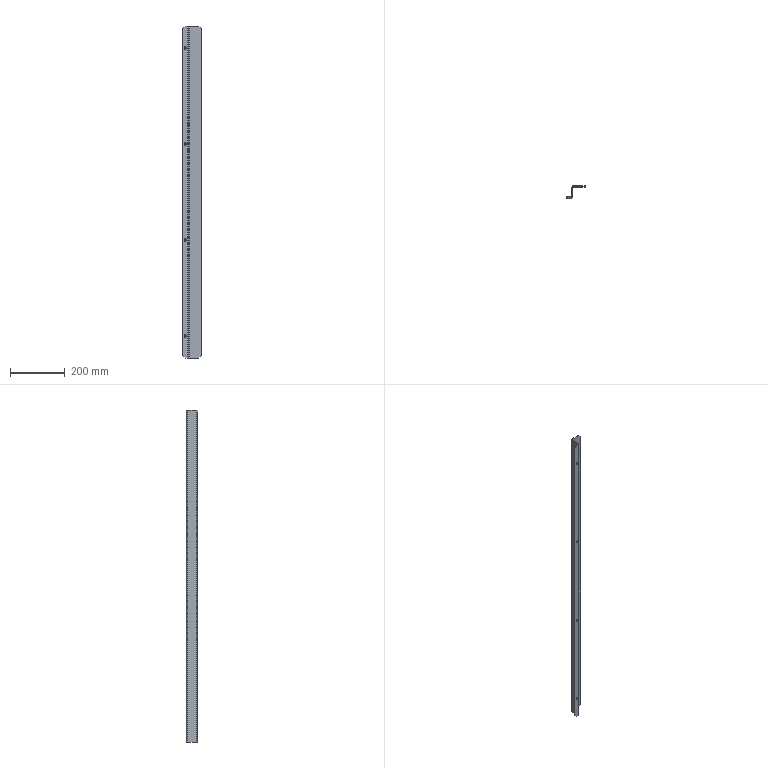Part | STEP file | HXGR200008-05-18 | 1 solid | 34 faces | box 70 x 42 x 1210 mm | volume 257088 mm3 | plane 22 | cylinder 12 | commonest cylinder face diameters 8 x8 6 x2 10 x2
STEP:
#1=CARTESIAN_POINT('',(10.,-2.,171.));
#2=VERTEX_POINT('',#1);
#3=CARTESIAN_POINT('',(10.,-2.,179.));
#4=VERTEX_POINT('',#3);
#5=CARTESIAN_POINT('',(10.,-2.,175.));
#6=DIRECTION('',(0.,1.,0.));
#7=DIRECTION('',(0.,0.,1.));
#8=AXIS2_PLACEMENT_3D('',#5,#6,#7);
#9=CIRCLE('',#8,4.);
#10=EDGE_CURVE('',#2,#4,#9,.T.);
#11=ORIENTED_EDGE('',*,*,#10,.F.);
#12=CARTESIAN_POINT('',(10.,0.,171.));
#13=VERTEX_POINT('',#12);
#14=CARTESIAN_POINT('',(10.,0.,171.));
#15=DIRECTION('',(0.,1.,0.));
#16=VECTOR('',#15,1000.);
#17=LINE('',#14,#16);
#18=EDGE_CURVE('',#2,#13,#17,.T.);
#19=ORIENTED_EDGE('',*,*,#18,.T.);
#20=CARTESIAN_POINT('',(10.,0.,179.));
#21=VERTEX_POINT('',#20);
#22=CARTESIAN_POINT('',(10.,0.,175.));
#23=DIRECTION('',(0.,1.,0.));
#24=DIRECTION('',(0.,0.,1.));
#25=AXIS2_PLACEMENT_3D('',#22,#23,#24);
#26=CIRCLE('',#25,4.);
#27=EDGE_CURVE('',#13,#21,#26,.T.);
#28=ORIENTED_EDGE('',*,*,#27,.T.);
#29=CARTESIAN_POINT('',(10.,0.,179.));
#30=DIRECTION('',(0.,1.,0.));
#31=VECTOR('',#30,1000.);
#32=LINE('',#29,#31);
#33=EDGE_CURVE('',#4,#21,#32,.T.);
#34=ORIENTED_EDGE('',*,*,#33,.F.);
#35=EDGE_LOOP('',(#11,#19,#28,#34));
#36=FACE_OUTER_BOUND('',#35,.T.);
#37=CARTESIAN_POINT('',(10.,0.,175.));
#38=DIRECTION('',(0.,1.,0.));
#39=DIRECTION('',(0.,0.,1.));
#40=AXIS2_PLACEMENT_3D('',#37,#38,#39);
#41=CYLINDRICAL_SURFACE('',#40,4.);
#42=ADVANCED_FACE('',(#36),#41,.F.);
#43=CARTESIAN_POINT('',(10.,-2.,-179.));
#44=VERTEX_POINT('',#43);
#45=CARTESIAN_POINT('',(10.,-2.,-171.));
#46=VERTEX_POINT('',#45);
#47=CARTESIAN_POINT('',(10.,-2.,-175.));
#48=DIRECTION('',(0.,1.,0.));
#49=DIRECTION('',(0.,0.,1.));
#50=AXIS2_PLACEMENT_3D('',#47,#48,#49);
#51=CIRCLE('',#50,4.);
#52=EDGE_CURVE('',#44,#46,#51,.T.);
#53=ORIENTED_EDGE('',*,*,#52,.F.);
#54=CARTESIAN_POINT('',(10.,0.,-179.));
#55=VERTEX_POINT('',#54);
#56=CARTESIAN_POINT('',(10.,0.,-179.));
#57=DIRECTION('',(0.,1.,0.));
#58=VECTOR('',#57,1000.);
#59=LINE('',#56,#58);
#60=EDGE_CURVE('',#44,#55,#59,.T.);
#61=ORIENTED_EDGE('',*,*,#60,.T.);
#62=CARTESIAN_POINT('',(10.,0.,-171.));
#63=VERTEX_POINT('',#62);
#64=CARTESIAN_POINT('',(10.,0.,-175.));
#65=DIRECTION('',(0.,1.,0.));
#66=DIRECTION('',(0.,0.,1.));
#67=AXIS2_PLACEMENT_3D('',#64,#65,#66);
#68=CIRCLE('',#67,4.);
#69=EDGE_CURVE('',#55,#63,#68,.T.);
#70=ORIENTED_EDGE('',*,*,#69,.T.);
#71=CARTESIAN_POINT('',(10.,0.,-171.));
#72=DIRECTION('',(0.,1.,0.));
#73=VECTOR('',#72,1000.);
#74=LINE('',#71,#73);
#75=EDGE_CURVE('',#46,#63,#74,.T.);
#76=ORIENTED_EDGE('',*,*,#75,.F.);
#77=EDGE_LOOP('',(#53,#61,#70,#76));
#78=FACE_OUTER_BOUND('',#77,.T.);
#79=CARTESIAN_POINT('',(10.,0.,-175.));
#80=DIRECTION('',(0.,1.,0.));
#81=DIRECTION('',(0.,0.,1.));
#82=AXIS2_PLACEMENT_3D('',#79,#80,#81);
#83=CYLINDRICAL_SURFACE('',#82,4.);
#84=ADVANCED_FACE('',(#78),#83,.F.);
#85=CARTESIAN_POINT('',(10.,-2.,521.));
#86=VERTEX_POINT('',#85);
#87=CARTESIAN_POINT('',(10.,-2.,529.));
#88=VERTEX_POINT('',#87);
#89=CARTESIAN_POINT('',(10.,-2.,525.));
#90=DIRECTION('',(0.,1.,0.));
#91=DIRECTION('',(0.,0.,1.));
#92=AXIS2_PLACEMENT_3D('',#89,#90,#91);
#93=CIRCLE('',#92,4.);
#94=EDGE_CURVE('',#86,#88,#93,.T.);
#95=ORIENTED_EDGE('',*,*,#94,.F.);
#96=CARTESIAN_POINT('',(10.,0.,521.));
#97=VERTEX_POINT('',#96);
#98=CARTESIAN_POINT('',(10.,0.,521.));
#99=DIRECTION('',(0.,1.,0.));
#100=VECTOR('',#99,1000.);
#101=LINE('',#98,#100);
#102=EDGE_CURVE('',#86,#97,#101,.T.);
#103=ORIENTED_EDGE('',*,*,#102,.T.);
#104=CARTESIAN_POINT('',(10.,0.,529.));
#105=VERTEX_POINT('',#104);
#106=CARTESIAN_POINT('',(10.,0.,525.));
#107=DIRECTION('',(0.,1.,0.));
#108=DIRECTION('',(0.,0.,1.));
#109=AXIS2_PLACEMENT_3D('',#106,#107,#108);
#110=CIRCLE('',#109,4.);
#111=EDGE_CURVE('',#97,#105,#110,.T.);
#112=ORIENTED_EDGE('',*,*,#111,.T.);
#113=CARTESIAN_POINT('',(10.,0.,529.));
#114=DIRECTION('',(0.,1.,0.));
#115=VECTOR('',#114,1000.);
#116=LINE('',#113,#115);
#117=EDGE_CURVE('',#88,#105,#116,.T.);
#118=ORIENTED_EDGE('',*,*,#117,.F.);
#119=EDGE_LOOP('',(#95,#103,#112,#118));
#120=FACE_OUTER_BOUND('',#119,.T.);
#121=CARTESIAN_POINT('',(10.,0.,525.));
#122=DIRECTION('',(0.,1.,0.));
#123=DIRECTION('',(0.,0.,1.));
#124=AXIS2_PLACEMENT_3D('',#121,#122,#123);
#125=CYLINDRICAL_SURFACE('',#124,4.);
#126=ADVANCED_FACE('',(#120),#125,.F.);
#127=CARTESIAN_POINT('',(10.,-2.,-529.));
#128=VERTEX_POINT('',#127);
#129=CARTESIAN_POINT('',(10.,-2.,-521.));
#130=VERTEX_POINT('',#129);
#131=CARTESIAN_POINT('',(10.,-2.,-525.));
#132=DIRECTION('',(0.,1.,0.));
#133=DIRECTION('',(0.,0.,1.));
#134=AXIS2_PLACEMENT_3D('',#131,#132,#133);
#135=CIRCLE('',#134,4.);
#136=EDGE_CURVE('',#128,#130,#135,.T.);
#137=ORIENTED_EDGE('',*,*,#136,.F.);
#138=CARTESIAN_POINT('',(10.,0.,-529.));
#139=VERTEX_POINT('',#138);
#140=CARTESIAN_POINT('',(10.,0.,-529.));
#141=DIRECTION('',(0.,1.,0.));
#142=VECTOR('',#141,1000.);
#143=LINE('',#140,#142);
#144=EDGE_CURVE('',#128,#139,#143,.T.);
#145=ORIENTED_EDGE('',*,*,#144,.T.);
#146=CARTESIAN_POINT('',(10.,0.,-521.));
#147=VERTEX_POINT('',#146);
#148=CARTESIAN_POINT('',(10.,0.,-525.));
#149=DIRECTION('',(0.,1.,0.));
#150=DIRECTION('',(0.,0.,1.));
#151=AXIS2_PLACEMENT_3D('',#148,#149,#150);
#152=CIRCLE('',#151,4.);
#153=EDGE_CURVE('',#139,#147,#152,.T.);
#154=ORIENTED_EDGE('',*,*,#153,.T.);
#155=CARTESIAN_POINT('',(10.,0.,-521.));
#156=DIRECTION('',(0.,1.,0.));
#157=VECTOR('',#156,1000.);
#158=LINE('',#155,#157);
#159=EDGE_CURVE('',#130,#147,#158,.T.);
#160=ORIENTED_EDGE('',*,*,#159,.F.);
#161=EDGE_LOOP('',(#137,#145,#154,#160));
#162=FACE_OUTER_BOUND('',#161,.T.);
#163=CARTESIAN_POINT('',(10.,0.,-525.));
#164=DIRECTION('',(0.,1.,0.));
#165=DIRECTION('',(0.,0.,1.));
#166=AXIS2_PLACEMENT_3D('',#163,#164,#165);
#167=CYLINDRICAL_SURFACE('',#166,4.);
#168=ADVANCED_FACE('',(#162),#167,.F.);
#169=CARTESIAN_POINT('',(20.,3.,605.));
#170=VERTEX_POINT('',#169);
#171=CARTESIAN_POINT('',(22.,3.,605.));
#172=VERTEX_POINT('',#171);
#173=CARTESIAN_POINT('',(20.,3.,605.));
#174=DIRECTION('',(1.,0.,0.));
#175=VECTOR('',#174,1000.);
#176=LINE('',#173,#175);
#177=EDGE_CURVE('',#170,#172,#176,.T.);
#178=ORIENTED_EDGE('',*,*,#177,.F.);
#179=CARTESIAN_POINT('',(17.,0.,605.));
#180=VERTEX_POINT('',#179);
#181=CARTESIAN_POINT('',(17.,3.,605.));
#182=DIRECTION('',(0.,0.,1.));
#183=DIRECTION('',(-1.,0.,0.));
#184=AXIS2_PLACEMENT_3D('',#181,#182,#183);
#185=CIRCLE('',#184,3.);
#186=EDGE_CURVE('',#180,#170,#185,.T.);
#187=ORIENTED_EDGE('',*,*,#186,.F.);
#188=CARTESIAN_POINT('',(17.,-2.,605.));
#189=VERTEX_POINT('',#188);
#190=CARTESIAN_POINT('',(17.,-2.,605.));
#191=DIRECTION('',(0.,1.,0.));
#192=VECTOR('',#191,1000.);
#193=LINE('',#190,#192);
#194=EDGE_CURVE('',#189,#180,#193,.T.);
#195=ORIENTED_EDGE('',*,*,#194,.F.);
#196=CARTESIAN_POINT('',(17.,3.,605.));
#197=DIRECTION('',(0.,0.,1.));
#198=DIRECTION('',(1.,0.,0.));
#199=AXIS2_PLACEMENT_3D('',#196,#197,#198);
#200=CIRCLE('',#199,5.);
#201=EDGE_CURVE('',#189,#172,#200,.T.);
#202=ORIENTED_EDGE('',*,*,#201,.T.);
#203=EDGE_LOOP('',(#178,#187,#195,#202));
#204=FACE_OUTER_BOUND('',#203,.T.);
#205=CARTESIAN_POINT('',(20.,3.,605.));
#206=DIRECTION('',(0.,0.,1.));
#207=DIRECTION('',(1.,0.,0.));
#208=AXIS2_PLACEMENT_3D('',#205,#206,#207);
#209=PLANE('',#208);
#210=ADVANCED_FACE('',(#204),#209,.T.);
#211=CARTESIAN_POINT('',(20.,35.,605.));
#212=VERTEX_POINT('',#211);
#213=CARTESIAN_POINT('',(20.,0.,605.));
#214=DIRECTION('',(0.,1.,0.));
#215=VECTOR('',#214,1000.);
#216=LINE('',#213,#215);
#217=EDGE_CURVE('',#170,#212,#216,.T.);
#218=ORIENTED_EDGE('',*,*,#217,.F.);
#219=ORIENTED_EDGE('',*,*,#177,.T.);
#220=CARTESIAN_POINT('',(22.,35.,605.));
#221=VERTEX_POINT('',#220);
#222=CARTESIAN_POINT('',(22.,0.,605.));
#223=DIRECTION('',(0.,1.,0.));
#224=VECTOR('',#223,1000.);
#225=LINE('',#222,#224);
#226=EDGE_CURVE('',#172,#221,#225,.T.);
#227=ORIENTED_EDGE('',*,*,#226,.T.);
#228=CARTESIAN_POINT('',(22.,35.,605.));
#229=DIRECTION('',(-1.,0.,0.));
#230=VECTOR('',#229,1000.);
#231=LINE('',#228,#230);
#232=EDGE_CURVE('',#221,#212,#231,.T.);
#233=ORIENTED_EDGE('',*,*,#232,.T.);
#234=EDGE_LOOP('',(#218,#219,#227,#233));
#235=FACE_OUTER_BOUND('',#234,.T.);
#236=CARTESIAN_POINT('',(17.,-2.,605.));
#237=DIRECTION('',(0.,0.,1.));
#238=DIRECTION('',(1.,0.,0.));
#239=AXIS2_PLACEMENT_3D('',#236,#237,#238);
#240=PLANE('',#239);
#241=ADVANCED_FACE('',(#235),#240,.T.);
#242=CARTESIAN_POINT('',(17.,0.,-605.));
#243=VERTEX_POINT('',#242);
#244=CARTESIAN_POINT('',(17.,-2.,-605.));
#245=VERTEX_POINT('',#244);
#246=CARTESIAN_POINT('',(17.,0.,-605.));
#247=DIRECTION('',(0.,-1.,0.));
#248=VECTOR('',#247,1000.);
#249=LINE('',#246,#248);
#250=EDGE_CURVE('',#243,#245,#249,.T.);
#251=ORIENTED_EDGE('',*,*,#250,.F.);
#252=CARTESIAN_POINT('',(20.,3.,-605.));
#253=VERTEX_POINT('',#252);
#254=CARTESIAN_POINT('',(17.,3.,-605.));
#255=DIRECTION('',(0.,0.,1.));
#256=DIRECTION('',(-1.,0.,0.));
#257=AXIS2_PLACEMENT_3D('',#254,#255,#256);
#258=CIRCLE('',#257,3.);
#259=EDGE_CURVE('',#243,#253,#258,.T.);
#260=ORIENTED_EDGE('',*,*,#259,.T.);
#261=CARTESIAN_POINT('',(22.,3.,-605.));
#262=VERTEX_POINT('',#261);
#263=CARTESIAN_POINT('',(22.,3.,-605.));
#264=DIRECTION('',(-1.,0.,0.));
#265=VECTOR('',#264,1000.);
#266=LINE('',#263,#265);
#267=EDGE_CURVE('',#262,#253,#266,.T.);
#268=ORIENTED_EDGE('',*,*,#267,.F.);
#269=CARTESIAN_POINT('',(17.,3.,-605.));
#270=DIRECTION('',(0.,0.,1.));
#271=DIRECTION('',(1.,0.,0.));
#272=AXIS2_PLACEMENT_3D('',#269,#270,#271);
#273=CIRCLE('',#272,5.);
#274=EDGE_CURVE('',#245,#262,#273,.T.);
#275=ORIENTED_EDGE('',*,*,#274,.F.);
#276=EDGE_LOOP('',(#251,#260,#268,#275));
#277=FACE_OUTER_BOUND('',#276,.T.);
#278=CARTESIAN_POINT('',(17.,0.,-605.));
#279=DIRECTION('',(0.,0.,-1.));
#280=DIRECTION('',(-1.,0.,0.));
#281=AXIS2_PLACEMENT_3D('',#278,#279,#280);
#282=PLANE('',#281);
#283=ADVANCED_FACE('',(#277),#282,.T.);
#284=CARTESIAN_POINT('',(10.,-2.,-605.));
#285=VERTEX_POINT('',#284);
#286=CARTESIAN_POINT('',(0.,-2.,-605.));
#287=DIRECTION('',(1.,0.,0.));
#288=VECTOR('',#287,1000.);
#289=LINE('',#286,#288);
#290=EDGE_CURVE('',#285,#245,#289,.T.);
#291=ORIENTED_EDGE('',*,*,#290,.F.);
#292=CARTESIAN_POINT('',(10.,0.,-605.));
#293=VERTEX_POINT('',#292);
#294=CARTESIAN_POINT('',(10.,3.,-605.));
#295=DIRECTION('',(0.,1.,0.));
#296=VECTOR('',#295,1000.);
#297=LINE('',#294,#296);
#298=EDGE_CURVE('',#285,#293,#297,.T.);
#299=ORIENTED_EDGE('',*,*,#298,.T.);
#300=CARTESIAN_POINT('',(0.,0.,-605.));
#301=DIRECTION('',(1.,0.,0.));
#302=VECTOR('',#301,1000.);
#303=LINE('',#300,#302);
#304=EDGE_CURVE('',#293,#243,#303,.T.);
#305=ORIENTED_EDGE('',*,*,#304,.T.);
#306=ORIENTED_EDGE('',*,*,#250,.T.);
#307=EDGE_LOOP('',(#291,#299,#305,#306));
#308=FACE_OUTER_BOUND('',#307,.T.);
#309=CARTESIAN_POINT('',(22.,3.,-605.));
#310=DIRECTION('',(0.,0.,-1.));
#311=DIRECTION('',(-1.,0.,0.));
#312=AXIS2_PLACEMENT_3D('',#309,#310,#311);
#313=PLANE('',#312);
#314=ADVANCED_FACE('',(#308),#313,.T.);
#315=CARTESIAN_POINT('',(25.,40.,605.));
#316=VERTEX_POINT('',#315);
#317=CARTESIAN_POINT('',(25.,38.,605.));
#318=VERTEX_POINT('',#317);
#319=CARTESIAN_POINT('',(25.,40.,605.));
#320=DIRECTION('',(0.,-1.,0.));
#321=VECTOR('',#320,1000.);
#322=LINE('',#319,#321);
#323=EDGE_CURVE('',#316,#318,#322,.T.);
#324=ORIENTED_EDGE('',*,*,#323,.F.);
#325=CARTESIAN_POINT('',(25.,35.,605.));
#326=DIRECTION('',(0.,0.,-1.));
#327=DIRECTION('',(1.,0.,0.));
#328=AXIS2_PLACEMENT_3D('',#325,#326,#327);
#329=CIRCLE('',#328,5.);
#330=EDGE_CURVE('',#212,#316,#329,.T.);
#331=ORIENTED_EDGE('',*,*,#330,.F.);
#332=ORIENTED_EDGE('',*,*,#232,.F.);
#333=CARTESIAN_POINT('',(25.,35.,605.));
#334=DIRECTION('',(0.,0.,-1.));
#335=DIRECTION('',(1.,0.,0.));
#336=AXIS2_PLACEMENT_3D('',#333,#334,#335);
#337=CIRCLE('',#336,3.);
#338=EDGE_CURVE('',#221,#318,#337,.T.);
#339=ORIENTED_EDGE('',*,*,#338,.T.);
#340=EDGE_LOOP('',(#324,#331,#332,#339));
#341=FACE_OUTER_BOUND('',#340,.T.);
#342=CARTESIAN_POINT('',(25.,40.,605.));
#343=DIRECTION('',(0.,0.,1.));
#344=DIRECTION('',(1.,0.,0.));
#345=AXIS2_PLACEMENT_3D('',#342,#343,#344);
#346=PLANE('',#345);
#347=ADVANCED_FACE('',(#341),#346,.T.);
#348=CARTESIAN_POINT('',(60.,38.,605.));
#349=VERTEX_POINT('',#348);
#350=CARTESIAN_POINT('',(20.,38.,605.));
#351=DIRECTION('',(1.,0.,0.));
#352=VECTOR('',#351,1000.);
#353=LINE('',#350,#352);
#354=EDGE_CURVE('',#318,#349,#353,.T.);
#355=ORIENTED_EDGE('',*,*,#354,.T.);
#356=CARTESIAN_POINT('',(60.,40.,605.));
#357=VERTEX_POINT('',#356);
#358=CARTESIAN_POINT('',(60.,35.,605.));
#359=DIRECTION('',(0.,1.,0.));
#360=VECTOR('',#359,1000.);
#361=LINE('',#358,#360);
#362=EDGE_CURVE('',#349,#357,#361,.T.);
#363=ORIENTED_EDGE('',*,*,#362,.T.);
#364=CARTESIAN_POINT('',(20.,40.,605.));
#365=DIRECTION('',(1.,0.,0.));
#366=VECTOR('',#365,1000.);
#367=LINE('',#364,#366);
#368=EDGE_CURVE('',#316,#357,#367,.T.);
#369=ORIENTED_EDGE('',*,*,#368,.F.);
#370=ORIENTED_EDGE('',*,*,#323,.T.);
#371=EDGE_LOOP('',(#355,#363,#369,#370));
#372=FACE_OUTER_BOUND('',#371,.T.);
#373=CARTESIAN_POINT('',(22.,35.,605.));
#374=DIRECTION('',(0.,0.,1.));
#375=DIRECTION('',(1.,0.,0.));
#376=AXIS2_PLACEMENT_3D('',#373,#374,#375);
#377=PLANE('',#376);
#378=ADVANCED_FACE('',(#372),#377,.T.);
#379=CARTESIAN_POINT('',(20.,35.,-605.));
#380=VERTEX_POINT('',#379);
#381=CARTESIAN_POINT('',(22.,35.,-605.));
#382=VERTEX_POINT('',#381);
#383=CARTESIAN_POINT('',(20.,35.,-605.));
#384=DIRECTION('',(1.,0.,0.));
#385=VECTOR('',#384,1000.);
#386=LINE('',#383,#385);
#387=EDGE_CURVE('',#380,#382,#386,.T.);
#388=ORIENTED_EDGE('',*,*,#387,.F.);
#389=CARTESIAN_POINT('',(25.,40.,-605.));
#390=VERTEX_POINT('',#389);
#391=CARTESIAN_POINT('',(25.,35.,-605.));
#392=DIRECTION('',(0.,0.,-1.));
#393=DIRECTION('',(1.,0.,0.));
#394=AXIS2_PLACEMENT_3D('',#391,#392,#393);
#395=CIRCLE('',#394,5.);
#396=EDGE_CURVE('',#380,#390,#395,.T.);
#397=ORIENTED_EDGE('',*,*,#396,.T.);
#398=CARTESIAN_POINT('',(25.,38.,-605.));
#399=VERTEX_POINT('',#398);
#400=CARTESIAN_POINT('',(25.,38.,-605.));
#401=DIRECTION('',(0.,1.,0.));
#402=VECTOR('',#401,1000.);
#403=LINE('',#400,#402);
#404=EDGE_CURVE('',#399,#390,#403,.T.);
#405=ORIENTED_EDGE('',*,*,#404,.F.);
#406=CARTESIAN_POINT('',(25.,35.,-605.));
#407=DIRECTION('',(0.,0.,-1.));
#408=DIRECTION('',(1.,0.,0.));
#409=AXIS2_PLACEMENT_3D('',#406,#407,#408);
#410=CIRCLE('',#409,3.);
#411=EDGE_CURVE('',#382,#399,#410,.T.);
#412=ORIENTED_EDGE('',*,*,#411,.F.);
#413=EDGE_LOOP('',(#388,#397,#405,#412));
#414=FACE_OUTER_BOUND('',#413,.T.);
#415=CARTESIAN_POINT('',(20.,35.,-605.));
#416=DIRECTION('',(0.,0.,-1.));
#417=DIRECTION('',(-1.,0.,0.));
#418=AXIS2_PLACEMENT_3D('',#415,#416,#417);
#419=PLANE('',#418);
#420=ADVANCED_FACE('',(#414),#419,.T.);
#421=CARTESIAN_POINT('',(20.,0.,-605.));
#422=DIRECTION('',(0.,1.,0.));
#423=VECTOR('',#422,1000.);
#424=LINE('',#421,#423);
#425=EDGE_CURVE('',#253,#380,#424,.T.);
#426=ORIENTED_EDGE('',*,*,#425,.T.);
#427=ORIENTED_EDGE('',*,*,#387,.T.);
#428=CARTESIAN_POINT('',(22.,0.,-605.));
#429=DIRECTION('',(0.,1.,0.));
#430=VECTOR('',#429,1000.);
#431=LINE('',#428,#430);
#432=EDGE_CURVE('',#262,#382,#431,.T.);
#433=ORIENTED_EDGE('',*,*,#432,.F.);
#434=ORIENTED_EDGE('',*,*,#267,.T.);
#435=EDGE_LOOP('',(#426,#427,#433,#434));
#436=FACE_OUTER_BOUND('',#435,.T.);
#437=CARTESIAN_POINT('',(25.,38.,-605.));
#438=DIRECTION('',(0.,0.,-1.));
#439=DIRECTION('',(-1.,0.,0.));
#440=AXIS2_PLACEMENT_3D('',#437,#438,#439);
#441=PLANE('',#440);
#442=ADVANCED_FACE('',(#436),#441,.T.);
#443=CARTESIAN_POINT('',(70.,38.,595.));
#444=VERTEX_POINT('',#443);
#445=CARTESIAN_POINT('',(70.,38.,-595.));
#446=VERTEX_POINT('',#445);
#447=CARTESIAN_POINT('',(70.,38.,605.));
#448=DIRECTION('',(0.,0.,-1.));
#449=VECTOR('',#448,1000.);
#450=LINE('',#447,#449);
#451=EDGE_CURVE('',#444,#446,#450,.T.);
#452=ORIENTED_EDGE('',*,*,#451,.F.);
#453=CARTESIAN_POINT('',(70.,38.,595.));
#454=DIRECTION('',(-0.7071,0.,0.7071));
#455=VECTOR('',#454,1000.);
#456=LINE('',#453,#455);
#457=EDGE_CURVE('',#444,#349,#456,.T.);
#458=ORIENTED_EDGE('',*,*,#457,.T.);
#459=ORIENTED_EDGE('',*,*,#354,.F.);
#460=CARTESIAN_POINT('',(25.,38.,605.));
#461=DIRECTION('',(0.,0.,-1.));
#462=VECTOR('',#461,1000.);
#463=LINE('',#460,#462);
#464=EDGE_CURVE('',#318,#399,#463,.T.);
#465=ORIENTED_EDGE('',*,*,#464,.T.);
#466=CARTESIAN_POINT('',(60.,38.,-605.));
#467=VERTEX_POINT('',#466);
#468=CARTESIAN_POINT('',(20.,38.,-605.));
#469=DIRECTION('',(1.,0.,0.));
#470=VECTOR('',#469,1000.);
#471=LINE('',#468,#470);
#472=EDGE_CURVE('',#399,#467,#471,.T.);
#473=ORIENTED_EDGE('',*,*,#472,.T.);
#474=CARTESIAN_POINT('',(60.,38.,-605.));
#475=DIRECTION('',(0.7071,0.,0.7071));
#476=VECTOR('',#475,1000.);
#477=LINE('',#474,#476);
#478=EDGE_CURVE('',#467,#446,#477,.T.);
#479=ORIENTED_EDGE('',*,*,#478,.T.);
#480=EDGE_LOOP('',(#452,#458,#459,#465,#473,#479));
#481=FACE_OUTER_BOUND('',#480,.T.);
#482=CARTESIAN_POINT('',(20.,38.,605.));
#483=DIRECTION('',(0.,1.,0.));
#484=DIRECTION('',(0.,0.,1.));
#485=AXIS2_PLACEMENT_3D('',#482,#483,#484);
#486=PLANE('',#485);
#487=ADVANCED_FACE('',(#481),#486,.F.);
#488=CARTESIAN_POINT('',(70.,40.,595.));
#489=VERTEX_POINT('',#488);
#490=CARTESIAN_POINT('',(70.,40.,-595.));
#491=VERTEX_POINT('',#490);
#492=CARTESIAN_POINT('',(70.,40.,605.));
#493=DIRECTION('',(0.,0.,-1.));
#494=VECTOR('',#493,1000.);
#495=LINE('',#492,#494);
#496=EDGE_CURVE('',#489,#491,#495,.T.);
#497=ORIENTED_EDGE('',*,*,#496,.F.);
#498=CARTESIAN_POINT('',(70.,40.,595.));
#499=DIRECTION('',(0.,-1.,0.));
#500=VECTOR('',#499,1000.);
#501=LINE('',#498,#500);
#502=EDGE_CURVE('',#489,#444,#501,.T.);
#503=ORIENTED_EDGE('',*,*,#502,.T.);
#504=ORIENTED_EDGE('',*,*,#451,.T.);
#505=CARTESIAN_POINT('',(70.,40.,-595.));
#506=DIRECTION('',(0.,1.,0.));
#507=VECTOR('',#506,1000.);
#508=LINE('',#505,#507);
#509=EDGE_CURVE('',#446,#491,#508,.T.);
#510=ORIENTED_EDGE('',*,*,#509,.T.);
#511=EDGE_LOOP('',(#497,#503,#504,#510));
#512=FACE_OUTER_BOUND('',#511,.T.);
#513=CARTESIAN_POINT('',(70.,40.,605.));
#514=DIRECTION('',(1.,0.,0.));
#515=DIRECTION('',(0.,0.,-1.));
#516=AXIS2_PLACEMENT_3D('',#513,#514,#515);
#517=PLANE('',#516);
#518=ADVANCED_FACE('',(#512),#517,.T.);
#519=ORIENTED_EDGE('',*,*,#368,.T.);
#520=CARTESIAN_POINT('',(40.,40.,625.));
#521=DIRECTION('',(0.7071,0.,-0.7071));
#522=VECTOR('',#521,1000.);
#523=LINE('',#520,#522);
#524=EDGE_CURVE('',#357,#489,#523,.T.);
#525=ORIENTED_EDGE('',*,*,#524,.T.);
#526=ORIENTED_EDGE('',*,*,#496,.T.);
#527=CARTESIAN_POINT('',(60.,40.,-605.));
#528=VERTEX_POINT('',#527);
#529=CARTESIAN_POINT('',(645.,40.,-20.));
#530=DIRECTION('',(-0.7071,0.,-0.7071));
#531=VECTOR('',#530,1000.);
#532=LINE('',#529,#531);
#533=EDGE_CURVE('',#491,#528,#532,.T.);
#534=ORIENTED_EDGE('',*,*,#533,.T.);
#535=CARTESIAN_POINT('',(20.,40.,-605.));
#536=DIRECTION('',(1.,0.,0.));
#537=VECTOR('',#536,1000.);
#538=LINE('',#535,#537);
#539=EDGE_CURVE('',#390,#528,#538,.T.);
#540=ORIENTED_EDGE('',*,*,#539,.F.);
#541=CARTESIAN_POINT('',(25.,40.,605.));
#542=DIRECTION('',(0.,0.,-1.));
#543=VECTOR('',#542,1000.);
#544=LINE('',#541,#543);
#545=EDGE_CURVE('',#316,#390,#544,.T.);
#546=ORIENTED_EDGE('',*,*,#545,.F.);
#547=EDGE_LOOP('',(#519,#525,#526,#534,#540,#546));
#548=FACE_OUTER_BOUND('',#547,.T.);
#549=CARTESIAN_POINT('',(20.,40.,605.));
#550=DIRECTION('',(0.,1.,0.));
#551=DIRECTION('',(0.,0.,1.));
#552=AXIS2_PLACEMENT_3D('',#549,#550,#551);
#553=PLANE('',#552);
#554=ADVANCED_FACE('',(#548),#553,.T.);
#555=ORIENTED_EDGE('',*,*,#396,.F.);
#556=CARTESIAN_POINT('',(20.,35.,605.));
#557=DIRECTION('',(0.,0.,-1.));
#558=VECTOR('',#557,1000.);
#559=LINE('',#556,#558);
#560=EDGE_CURVE('',#212,#380,#559,.T.);
#561=ORIENTED_EDGE('',*,*,#560,.F.);
#562=ORIENTED_EDGE('',*,*,#330,.T.);
#563=ORIENTED_EDGE('',*,*,#545,.T.);
#564=EDGE_LOOP('',(#555,#561,#562,#563));
#565=FACE_OUTER_BOUND('',#564,.T.);
#566=CARTESIAN_POINT('',(25.,35.,605.));
#567=DIRECTION('',(0.,0.,-1.));
#568=DIRECTION('',(-1.,0.,0.));
#569=AXIS2_PLACEMENT_3D('',#566,#567,#568);
#570=CYLINDRICAL_SURFACE('',#569,5.);
#571=ADVANCED_FACE('',(#565),#570,.T.);
#572=ORIENTED_EDGE('',*,*,#425,.F.);
#573=CARTESIAN_POINT('',(20.,3.,605.));
#574=DIRECTION('',(0.,0.,-1.));
#575=VECTOR('',#574,1000.);
#576=LINE('',#573,#575);
#577=EDGE_CURVE('',#170,#253,#576,.T.);
#578=ORIENTED_EDGE('',*,*,#577,.F.);
#579=ORIENTED_EDGE('',*,*,#217,.T.);
#580=ORIENTED_EDGE('',*,*,#560,.T.);
#581=EDGE_LOOP('',(#572,#578,#579,#580));
#582=FACE_OUTER_BOUND('',#581,.T.);
#583=CARTESIAN_POINT('',(20.,0.,605.));
#584=DIRECTION('',(-1.,0.,0.));
#585=DIRECTION('',(0.,0.,1.));
#586=AXIS2_PLACEMENT_3D('',#583,#584,#585);
#587=PLANE('',#586);
#588=ADVANCED_FACE('',(#582),#587,.T.);
#589=ORIENTED_EDGE('',*,*,#259,.F.);
#590=CARTESIAN_POINT('',(17.,0.,605.));
#591=DIRECTION('',(0.,0.,-1.));
#592=VECTOR('',#591,1000.);
#593=LINE('',#590,#592);
#594=EDGE_CURVE('',#180,#243,#593,.T.);
#595=ORIENTED_EDGE('',*,*,#594,.F.);
#596=ORIENTED_EDGE('',*,*,#186,.T.);
#597=ORIENTED_EDGE('',*,*,#577,.T.);
#598=EDGE_LOOP('',(#589,#595,#596,#597));
#599=FACE_OUTER_BOUND('',#598,.T.);
#600=CARTESIAN_POINT('',(17.,3.,605.));
#601=DIRECTION('',(0.,0.,-1.));
#602=DIRECTION('',(-1.,0.,0.));
#603=AXIS2_PLACEMENT_3D('',#600,#601,#602);
#604=CYLINDRICAL_SURFACE('',#603,3.);
#605=ADVANCED_FACE('',(#599),#604,.F.);
#606=CARTESIAN_POINT('',(10.,0.,175.));
#607=DIRECTION('',(0.,1.,0.));
#608=DIRECTION('',(0.,0.,1.));
#609=AXIS2_PLACEMENT_3D('',#606,#607,#608);
#610=CIRCLE('',#609,4.);
#611=EDGE_CURVE('',#21,#13,#610,.T.);
#612=ORIENTED_EDGE('',*,*,#611,.F.);
#613=ORIENTED_EDGE('',*,*,#27,.F.);
#614=EDGE_LOOP('',(#612,#613));
#615=FACE_BOUND('',#614,.T.);
#616=CARTESIAN_POINT('',(10.,0.,-175.));
#617=DIRECTION('',(0.,1.,0.));
#618=DIRECTION('',(0.,0.,1.));
#619=AXIS2_PLACEMENT_3D('',#616,#617,#618);
#620=CIRCLE('',#619,4.);
#621=EDGE_CURVE('',#63,#55,#620,.T.);
#622=ORIENTED_EDGE('',*,*,#621,.F.);
#623=ORIENTED_EDGE('',*,*,#69,.F.);
#624=EDGE_LOOP('',(#622,#623));
#625=FACE_BOUND('',#624,.T.);
#626=CARTESIAN_POINT('',(10.,0.,525.));
#627=DIRECTION('',(0.,1.,0.));
#628=DIRECTION('',(0.,0.,1.));
#629=AXIS2_PLACEMENT_3D('',#626,#627,#628);
#630=CIRCLE('',#629,4.);
#631=EDGE_CURVE('',#105,#97,#630,.T.);
#632=ORIENTED_EDGE('',*,*,#631,.F.);
#633=ORIENTED_EDGE('',*,*,#111,.F.);
#634=EDGE_LOOP('',(#632,#633));
#635=FACE_BOUND('',#634,.T.);
#636=CARTESIAN_POINT('',(10.,0.,-525.));
#637=DIRECTION('',(0.,1.,0.));
#638=DIRECTION('',(0.,0.,1.));
#639=AXIS2_PLACEMENT_3D('',#636,#637,#638);
#640=CIRCLE('',#639,4.);
#641=EDGE_CURVE('',#147,#139,#640,.T.);
#642=ORIENTED_EDGE('',*,*,#641,.F.);
#643=ORIENTED_EDGE('',*,*,#153,.F.);
#644=EDGE_LOOP('',(#642,#643));
#645=FACE_BOUND('',#644,.T.);
#646=CARTESIAN_POINT('',(0.,0.,595.));
#647=VERTEX_POINT('',#646);
#648=CARTESIAN_POINT('',(0.,0.,-595.));
#649=VERTEX_POINT('',#648);
#650=CARTESIAN_POINT('',(0.,0.,605.));
#651=DIRECTION('',(0.,0.,-1.));
#652=VECTOR('',#651,1000.);
#653=LINE('',#650,#652);
#654=EDGE_CURVE('',#647,#649,#653,.T.);
#655=ORIENTED_EDGE('',*,*,#654,.F.);
#656=CARTESIAN_POINT('',(10.,0.,605.));
#657=VERTEX_POINT('',#656);
#658=CARTESIAN_POINT('',(5.,0.,600.));
#659=DIRECTION('',(0.7071,0.,0.7071));
#660=VECTOR('',#659,1000.);
#661=LINE('',#658,#660);
#662=EDGE_CURVE('',#647,#657,#661,.T.);
#663=ORIENTED_EDGE('',*,*,#662,.T.);
#664=CARTESIAN_POINT('',(0.,0.,605.));
#665=DIRECTION('',(1.,0.,0.));
#666=VECTOR('',#665,1000.);
#667=LINE('',#664,#666);
#668=EDGE_CURVE('',#657,#180,#667,.T.);
#669=ORIENTED_EDGE('',*,*,#668,.T.);
#670=ORIENTED_EDGE('',*,*,#594,.T.);
#671=ORIENTED_EDGE('',*,*,#304,.F.);
#672=CARTESIAN_POINT('',(-600.,0.,5.));
#673=DIRECTION('',(-0.7071,0.,0.7071));
#674=VECTOR('',#673,1000.);
#675=LINE('',#672,#674);
#676=EDGE_CURVE('',#293,#649,#675,.T.);
#677=ORIENTED_EDGE('',*,*,#676,.T.);
#678=EDGE_LOOP('',(#655,#663,#669,#670,#671,#677));
#679=FACE_OUTER_BOUND('',#678,.T.);
#680=CARTESIAN_POINT('',(0.,0.,605.));
#681=DIRECTION('',(0.,1.,0.));
#682=DIRECTION('',(0.,0.,1.));
#683=AXIS2_PLACEMENT_3D('',#680,#681,#682);
#684=PLANE('',#683);
#685=ADVANCED_FACE('',(#615,#625,#635,#645,#679),#684,.T.);
#686=CARTESIAN_POINT('',(0.,-2.,595.));
#687=VERTEX_POINT('',#686);
#688=CARTESIAN_POINT('',(0.,-2.,-595.));
#689=VERTEX_POINT('',#688);
#690=CARTESIAN_POINT('',(0.,-2.,605.));
#691=DIRECTION('',(0.,0.,-1.));
#692=VECTOR('',#691,1000.);
#693=LINE('',#690,#692);
#694=EDGE_CURVE('',#687,#689,#693,.T.);
#695=ORIENTED_EDGE('',*,*,#694,.F.);
#696=CARTESIAN_POINT('',(0.,-2.,595.));
#697=DIRECTION('',(0.,1.,0.));
#698=VECTOR('',#697,1000.);
#699=LINE('',#696,#698);
#700=EDGE_CURVE('',#687,#647,#699,.T.);
#701=ORIENTED_EDGE('',*,*,#700,.T.);
#702=ORIENTED_EDGE('',*,*,#654,.T.);
#703=CARTESIAN_POINT('',(0.,-2.,-595.));
#704=DIRECTION('',(0.,-1.,0.));
#705=VECTOR('',#704,1000.);
#706=LINE('',#703,#705);
#707=EDGE_CURVE('',#649,#689,#706,.T.);
#708=ORIENTED_EDGE('',*,*,#707,.T.);
#709=EDGE_LOOP('',(#695,#701,#702,#708));
#710=FACE_OUTER_BOUND('',#709,.T.);
#711=CARTESIAN_POINT('',(0.,-2.,605.));
#712=DIRECTION('',(-1.,0.,0.));
#713=DIRECTION('',(0.,0.,1.));
#714=AXIS2_PLACEMENT_3D('',#711,#712,#713);
#715=PLANE('',#714);
#716=ADVANCED_FACE('',(#710),#715,.T.);
#717=CARTESIAN_POINT('',(10.,-2.,175.));
#718=DIRECTION('',(0.,1.,0.));
#719=DIRECTION('',(0.,0.,1.));
#720=AXIS2_PLACEMENT_3D('',#717,#718,#719);
#721=CIRCLE('',#720,4.);
#722=EDGE_CURVE('',#4,#2,#721,.T.);
#723=ORIENTED_EDGE('',*,*,#722,.T.);
#724=ORIENTED_EDGE('',*,*,#10,.T.);
#725=EDGE_LOOP('',(#723,#724));
#726=FACE_BOUND('',#725,.T.);
#727=CARTESIAN_POINT('',(10.,-2.,-175.));
#728=DIRECTION('',(0.,1.,0.));
#729=DIRECTION('',(0.,0.,1.));
#730=AXIS2_PLACEMENT_3D('',#727,#728,#729);
#731=CIRCLE('',#730,4.);
#732=EDGE_CURVE('',#46,#44,#731,.T.);
#733=ORIENTED_EDGE('',*,*,#732,.T.);
#734=ORIENTED_EDGE('',*,*,#52,.T.);
#735=EDGE_LOOP('',(#733,#734));
#736=FACE_BOUND('',#735,.T.);
#737=CARTESIAN_POINT('',(10.,-2.,525.));
#738=DIRECTION('',(0.,1.,0.));
#739=DIRECTION('',(0.,0.,1.));
#740=AXIS2_PLACEMENT_3D('',#737,#738,#739);
#741=CIRCLE('',#740,4.);
#742=EDGE_CURVE('',#88,#86,#741,.T.);
#743=ORIENTED_EDGE('',*,*,#742,.T.);
#744=ORIENTED_EDGE('',*,*,#94,.T.);
#745=EDGE_LOOP('',(#743,#744));
#746=FACE_BOUND('',#745,.T.);
#747=CARTESIAN_POINT('',(10.,-2.,-525.));
#748=DIRECTION('',(0.,1.,0.));
#749=DIRECTION('',(0.,0.,1.));
#750=AXIS2_PLACEMENT_3D('',#747,#748,#749);
#751=CIRCLE('',#750,4.);
#752=EDGE_CURVE('',#130,#128,#751,.T.);
#753=ORIENTED_EDGE('',*,*,#752,.T.);
#754=ORIENTED_EDGE('',*,*,#136,.T.);
#755=EDGE_LOOP('',(#753,#754));
#756=FACE_BOUND('',#755,.T.);
#757=CARTESIAN_POINT('',(10.,-2.,605.));
#758=VERTEX_POINT('',#757);
#759=CARTESIAN_POINT('',(0.,-2.,605.));
#760=DIRECTION('',(1.,0.,0.));
#761=VECTOR('',#760,1000.);
#762=LINE('',#759,#761);
#763=EDGE_CURVE('',#758,#189,#762,.T.);
#764=ORIENTED_EDGE('',*,*,#763,.F.);
#765=CARTESIAN_POINT('',(0.,-2.,595.));
#766=DIRECTION('',(-0.7071,0.,-0.7071));
#767=VECTOR('',#766,1000.);
#768=LINE('',#765,#767);
#769=EDGE_CURVE('',#758,#687,#768,.T.);
#770=ORIENTED_EDGE('',*,*,#769,.T.);
#771=ORIENTED_EDGE('',*,*,#694,.T.);
#772=CARTESIAN_POINT('',(10.,-2.,-605.));
#773=DIRECTION('',(0.7071,0.,-0.7071));
#774=VECTOR('',#773,1000.);
#775=LINE('',#772,#774);
#776=EDGE_CURVE('',#689,#285,#775,.T.);
#777=ORIENTED_EDGE('',*,*,#776,.T.);
#778=ORIENTED_EDGE('',*,*,#290,.T.);
#779=CARTESIAN_POINT('',(17.,-2.,605.));
#780=DIRECTION('',(0.,0.,-1.));
#781=VECTOR('',#780,1000.);
#782=LINE('',#779,#781);
#783=EDGE_CURVE('',#189,#245,#782,.T.);
#784=ORIENTED_EDGE('',*,*,#783,.F.);
#785=EDGE_LOOP('',(#764,#770,#771,#777,#778,#784));
#786=FACE_OUTER_BOUND('',#785,.T.);
#787=CARTESIAN_POINT('',(0.,-2.,605.));
#788=DIRECTION('',(0.,1.,0.));
#789=DIRECTION('',(0.,0.,1.));
#790=AXIS2_PLACEMENT_3D('',#787,#788,#789);
#791=PLANE('',#790);
#792=ADVANCED_FACE('',(#726,#736,#746,#756,#786),#791,.F.);
#793=ORIENTED_EDGE('',*,*,#274,.T.);
#794=CARTESIAN_POINT('',(22.,3.,605.));
#795=DIRECTION('',(0.,0.,-1.));
#796=VECTOR('',#795,1000.);
#797=LINE('',#794,#796);
#798=EDGE_CURVE('',#172,#262,#797,.T.);
#799=ORIENTED_EDGE('',*,*,#798,.F.);
#800=ORIENTED_EDGE('',*,*,#201,.F.);
#801=ORIENTED_EDGE('',*,*,#783,.T.);
#802=EDGE_LOOP('',(#793,#799,#800,#801));
#803=FACE_OUTER_BOUND('',#802,.T.);
#804=CARTESIAN_POINT('',(17.,3.,605.));
#805=DIRECTION('',(0.,0.,-1.));
#806=DIRECTION('',(-1.,0.,0.));
#807=AXIS2_PLACEMENT_3D('',#804,#805,#806);
#808=CYLINDRICAL_SURFACE('',#807,5.);
#809=ADVANCED_FACE('',(#803),#808,.T.);
#810=ORIENTED_EDGE('',*,*,#432,.T.);
#811=CARTESIAN_POINT('',(22.,35.,605.));
#812=DIRECTION('',(0.,0.,-1.));
#813=VECTOR('',#812,1000.);
#814=LINE('',#811,#813);
#815=EDGE_CURVE('',#221,#382,#814,.T.);
#816=ORIENTED_EDGE('',*,*,#815,.F.);
#817=ORIENTED_EDGE('',*,*,#226,.F.);
#818=ORIENTED_EDGE('',*,*,#798,.T.);
#819=EDGE_LOOP('',(#810,#816,#817,#818));
#820=FACE_OUTER_BOUND('',#819,.T.);
#821=CARTESIAN_POINT('',(22.,0.,605.));
#822=DIRECTION('',(-1.,0.,0.));
#823=DIRECTION('',(0.,0.,1.));
#824=AXIS2_PLACEMENT_3D('',#821,#822,#823);
#825=PLANE('',#824);
#826=ADVANCED_FACE('',(#820),#825,.F.);
#827=ORIENTED_EDGE('',*,*,#411,.T.);
#828=ORIENTED_EDGE('',*,*,#464,.F.);
#829=ORIENTED_EDGE('',*,*,#338,.F.);
#830=ORIENTED_EDGE('',*,*,#815,.T.);
#831=EDGE_LOOP('',(#827,#828,#829,#830));
#832=FACE_OUTER_BOUND('',#831,.T.);
#833=CARTESIAN_POINT('',(25.,35.,605.));
#834=DIRECTION('',(0.,0.,-1.));
#835=DIRECTION('',(-1.,0.,0.));
#836=AXIS2_PLACEMENT_3D('',#833,#834,#835);
#837=CYLINDRICAL_SURFACE('',#836,3.);
#838=ADVANCED_FACE('',(#832),#837,.F.);
#839=ORIENTED_EDGE('',*,*,#668,.F.);
#840=CARTESIAN_POINT('',(10.,35.,605.));
#841=DIRECTION('',(0.,-1.,0.));
#842=VECTOR('',#841,1000.);
#843=LINE('',#840,#842);
#844=EDGE_CURVE('',#657,#758,#843,.T.);
#845=ORIENTED_EDGE('',*,*,#844,.T.);
#846=ORIENTED_EDGE('',*,*,#763,.T.);
#847=ORIENTED_EDGE('',*,*,#194,.T.);
#848=EDGE_LOOP('',(#839,#845,#846,#847));
#849=FACE_OUTER_BOUND('',#848,.T.);
#850=CARTESIAN_POINT('',(25.,35.,605.));
#851=DIRECTION('',(0.,0.,1.));
#852=DIRECTION('',(1.,0.,0.));
#853=AXIS2_PLACEMENT_3D('',#850,#851,#852);
#854=PLANE('',#853);
#855=ADVANCED_FACE('',(#849),#854,.T.);
#856=ORIENTED_EDGE('',*,*,#539,.T.);
#857=CARTESIAN_POINT('',(60.,38.,-605.));
#858=DIRECTION('',(0.,-1.,0.));
#859=VECTOR('',#858,1000.);
#860=LINE('',#857,#859);
#861=EDGE_CURVE('',#528,#467,#860,.T.);
#862=ORIENTED_EDGE('',*,*,#861,.T.);
#863=ORIENTED_EDGE('',*,*,#472,.F.);
#864=ORIENTED_EDGE('',*,*,#404,.T.);
#865=EDGE_LOOP('',(#856,#862,#863,#864));
#866=FACE_OUTER_BOUND('',#865,.T.);
#867=CARTESIAN_POINT('',(25.,35.,-605.));
#868=DIRECTION('',(0.,0.,1.));
#869=DIRECTION('',(1.,0.,0.));
#870=AXIS2_PLACEMENT_3D('',#867,#868,#869);
#871=PLANE('',#870);
#872=ADVANCED_FACE('',(#866),#871,.F.);
#873=ORIENTED_EDGE('',*,*,#144,.F.);
#874=ORIENTED_EDGE('',*,*,#752,.F.);
#875=ORIENTED_EDGE('',*,*,#159,.T.);
#876=ORIENTED_EDGE('',*,*,#641,.T.);
#877=EDGE_LOOP('',(#873,#874,#875,#876));
#878=FACE_OUTER_BOUND('',#877,.T.);
#879=CARTESIAN_POINT('',(10.,0.,-525.));
#880=DIRECTION('',(0.,1.,0.));
#881=DIRECTION('',(0.,0.,1.));
#882=AXIS2_PLACEMENT_3D('',#879,#880,#881);
#883=CYLINDRICAL_SURFACE('',#882,4.);
#884=ADVANCED_FACE('',(#878),#883,.F.);
#885=ORIENTED_EDGE('',*,*,#102,.F.);
#886=ORIENTED_EDGE('',*,*,#742,.F.);
#887=ORIENTED_EDGE('',*,*,#117,.T.);
#888=ORIENTED_EDGE('',*,*,#631,.T.);
#889=EDGE_LOOP('',(#885,#886,#887,#888));
#890=FACE_OUTER_BOUND('',#889,.T.);
#891=CARTESIAN_POINT('',(10.,0.,525.));
#892=DIRECTION('',(0.,1.,0.));
#893=DIRECTION('',(0.,0.,1.));
#894=AXIS2_PLACEMENT_3D('',#891,#892,#893);
#895=CYLINDRICAL_SURFACE('',#894,4.);
#896=ADVANCED_FACE('',(#890),#895,.F.);
#897=ORIENTED_EDGE('',*,*,#60,.F.);
#898=ORIENTED_EDGE('',*,*,#732,.F.);
#899=ORIENTED_EDGE('',*,*,#75,.T.);
#900=ORIENTED_EDGE('',*,*,#621,.T.);
#901=EDGE_LOOP('',(#897,#898,#899,#900));
#902=FACE_OUTER_BOUND('',#901,.T.);
#903=CARTESIAN_POINT('',(10.,0.,-175.));
#904=DIRECTION('',(0.,1.,0.));
#905=DIRECTION('',(0.,0.,1.));
#906=AXIS2_PLACEMENT_3D('',#903,#904,#905);
#907=CYLINDRICAL_SURFACE('',#906,4.);
#908=ADVANCED_FACE('',(#902),#907,.F.);
#909=ORIENTED_EDGE('',*,*,#18,.F.);
#910=ORIENTED_EDGE('',*,*,#722,.F.);
#911=ORIENTED_EDGE('',*,*,#33,.T.);
#912=ORIENTED_EDGE('',*,*,#611,.T.);
#913=EDGE_LOOP('',(#909,#910,#911,#912));
#914=FACE_OUTER_BOUND('',#913,.T.);
#915=CARTESIAN_POINT('',(10.,0.,175.));
#916=DIRECTION('',(0.,1.,0.));
#917=DIRECTION('',(0.,0.,1.));
#918=AXIS2_PLACEMENT_3D('',#915,#916,#917);
#919=CYLINDRICAL_SURFACE('',#918,4.);
#920=ADVANCED_FACE('',(#914),#919,.F.);
#921=ORIENTED_EDGE('',*,*,#524,.F.);
#922=ORIENTED_EDGE('',*,*,#362,.F.);
#923=ORIENTED_EDGE('',*,*,#457,.F.);
#924=ORIENTED_EDGE('',*,*,#502,.F.);
#925=EDGE_LOOP('',(#921,#922,#923,#924));
#926=FACE_OUTER_BOUND('',#925,.T.);
#927=CARTESIAN_POINT('',(70.,40.,595.));
#928=DIRECTION('',(-0.7071,0.,-0.7071));
#929=DIRECTION('',(0.,-1.,0.));
#930=AXIS2_PLACEMENT_3D('',#927,#928,#929);
#931=PLANE('',#930);
#932=ADVANCED_FACE('',(#926),#931,.F.);
#933=ORIENTED_EDGE('',*,*,#769,.F.);
#934=ORIENTED_EDGE('',*,*,#844,.F.);
#935=ORIENTED_EDGE('',*,*,#662,.F.);
#936=ORIENTED_EDGE('',*,*,#700,.F.);
#937=EDGE_LOOP('',(#933,#934,#935,#936));
#938=FACE_OUTER_BOUND('',#937,.T.);
#939=CARTESIAN_POINT('',(0.,-2.,595.));
#940=DIRECTION('',(0.7071,0.,-0.7071));
#941=DIRECTION('',(0.,1.,0.));
#942=AXIS2_PLACEMENT_3D('',#939,#940,#941);
#943=PLANE('',#942);
#944=ADVANCED_FACE('',(#938),#943,.F.);
#945=ORIENTED_EDGE('',*,*,#776,.F.);
#946=ORIENTED_EDGE('',*,*,#707,.F.);
#947=ORIENTED_EDGE('',*,*,#676,.F.);
#948=ORIENTED_EDGE('',*,*,#298,.F.);
#949=EDGE_LOOP('',(#945,#946,#947,#948));
#950=FACE_OUTER_BOUND('',#949,.T.);
#951=CARTESIAN_POINT('',(10.,3.,-605.));
#952=DIRECTION('',(0.7071,0.,0.7071));
#953=DIRECTION('',(0.,1.,0.));
#954=AXIS2_PLACEMENT_3D('',#951,#952,#953);
#955=PLANE('',#954);
#956=ADVANCED_FACE('',(#950),#955,.F.);
#957=ORIENTED_EDGE('',*,*,#533,.F.);
#958=ORIENTED_EDGE('',*,*,#509,.F.);
#959=ORIENTED_EDGE('',*,*,#478,.F.);
#960=ORIENTED_EDGE('',*,*,#861,.F.);
#961=EDGE_LOOP('',(#957,#958,#959,#960));
#962=FACE_OUTER_BOUND('',#961,.T.);
#963=CARTESIAN_POINT('',(60.,35.,-605.));
#964=DIRECTION('',(0.7071,0.,-0.7071));
#965=DIRECTION('',(0.,1.,0.));
#966=AXIS2_PLACEMENT_3D('',#963,#964,#965);
#967=PLANE('',#966);
#968=ADVANCED_FACE('',(#962),#967,.T.);
#969=CLOSED_SHELL('',(#42,#84,#126,#168,#210,#241,#283,#314,#347,#378,#420,#442,#487,#518,#554,#571,#588,#605,#685,#716,#792,#809,#826,#838,#855,#872,#884,#896,#908,#920,#932,#944,#956,#968));
#970=MANIFOLD_SOLID_BREP('',#969);
#971=CARTESIAN_POINT('',(0.,0.,0.));
#972=DIRECTION('',(0.,0.,1.));
#973=DIRECTION('',(1.,0.,0.));
#974=AXIS2_PLACEMENT_3D('',#971,#972,#973);
#975=(LENGTH_UNIT()NAMED_UNIT(*)SI_UNIT(.MILLI.,.METRE.));
#976=UNCERTAINTY_MEASURE_WITH_UNIT(LENGTH_MEASURE(0.00001),#975,'','');
#977=(NAMED_UNIT(*)PLANE_ANGLE_UNIT()SI_UNIT($,.RADIAN.));
#978=(NAMED_UNIT(*)SI_UNIT($,.STERADIAN.)SOLID_ANGLE_UNIT());
#979=(GEOMETRIC_REPRESENTATION_CONTEXT(3)GLOBAL_UNCERTAINTY_ASSIGNED_CONTEXT((#976))GLOBAL_UNIT_ASSIGNED_CONTEXT((#975,#977,#978))REPRESENTATION_CONTEXT('',''));
#980=ADVANCED_BREP_SHAPE_REPRESENTATION('',(#970,#974),#979);